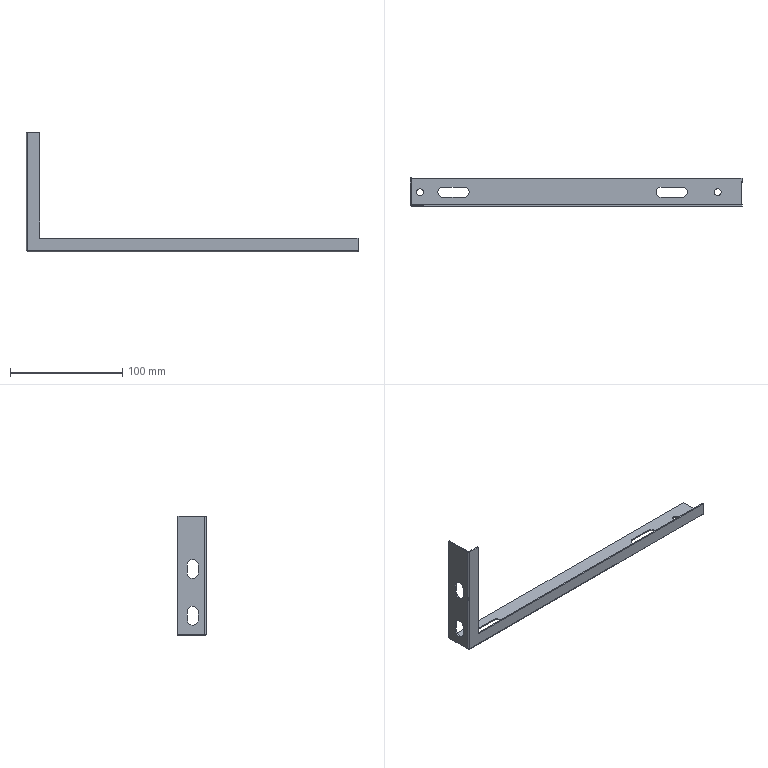Part | 1 solid | 44 faces | box 296 x 25 x 106.7 mm | volume 13427 mm3 | plane 28 | cylinder 16 | commonest cylinder face diameters 6 x4 9 x4 10 x4 0.4 x2 2.4 x2
STEP:
#1=CARTESIAN_POINT('',(125.7,14.5,-0.2));
#2=VERTEX_POINT('',#1);
#3=CARTESIAN_POINT('',(125.7,8.5,-0.2));
#4=VERTEX_POINT('',#3);
#5=CARTESIAN_POINT('',(125.7,11.5,-0.2));
#6=DIRECTION('',(0.,0.,1.));
#7=DIRECTION('',(0.,-1.,0.));
#8=AXIS2_PLACEMENT_3D('',#5,#6,#7);
#9=CIRCLE('',#8,3.);
#10=EDGE_CURVE('',#2,#4,#9,.T.);
#11=ORIENTED_EDGE('',*,*,#10,.T.);
#12=CARTESIAN_POINT('',(125.7,8.5,-1.2));
#13=VERTEX_POINT('',#12);
#14=CARTESIAN_POINT('',(125.7,8.5,8.8));
#15=DIRECTION('',(0.,0.,-1.));
#16=VECTOR('',#15,1000.);
#17=LINE('',#14,#16);
#18=EDGE_CURVE('',#4,#13,#17,.T.);
#19=ORIENTED_EDGE('',*,*,#18,.T.);
#20=CARTESIAN_POINT('',(125.7,14.5,-1.2));
#21=VERTEX_POINT('',#20);
#22=CARTESIAN_POINT('',(125.7,11.5,-1.2));
#23=DIRECTION('',(0.,0.,-1.));
#24=DIRECTION('',(0.,1.,0.));
#25=AXIS2_PLACEMENT_3D('',#22,#23,#24);
#26=CIRCLE('',#25,3.);
#27=EDGE_CURVE('',#13,#21,#26,.T.);
#28=ORIENTED_EDGE('',*,*,#27,.T.);
#29=CARTESIAN_POINT('',(125.7,14.5,8.8));
#30=DIRECTION('',(0.,0.,-1.));
#31=VECTOR('',#30,1000.);
#32=LINE('',#29,#31);
#33=EDGE_CURVE('',#2,#21,#32,.T.);
#34=ORIENTED_EDGE('',*,*,#33,.F.);
#35=EDGE_LOOP('',(#11,#19,#28,#34));
#36=FACE_OUTER_BOUND('',#35,.T.);
#37=CARTESIAN_POINT('',(125.7,11.5,8.8));
#38=DIRECTION('',(0.,0.,-1.));
#39=DIRECTION('',(0.,1.,0.));
#40=AXIS2_PLACEMENT_3D('',#37,#38,#39);
#41=CYLINDRICAL_SURFACE('',#40,3.);
#42=ADVANCED_FACE('',(#36),#41,.F.);
#43=CARTESIAN_POINT('',(-139.8,14.5,-0.2));
#44=VERTEX_POINT('',#43);
#45=CARTESIAN_POINT('',(-139.8,8.5,-0.2));
#46=VERTEX_POINT('',#45);
#47=CARTESIAN_POINT('',(-139.8,11.5,-0.2));
#48=DIRECTION('',(0.,0.,1.));
#49=DIRECTION('',(0.,-1.,0.));
#50=AXIS2_PLACEMENT_3D('',#47,#48,#49);
#51=CIRCLE('',#50,3.);
#52=EDGE_CURVE('',#44,#46,#51,.T.);
#53=ORIENTED_EDGE('',*,*,#52,.T.);
#54=CARTESIAN_POINT('',(-139.8,8.5,-1.2));
#55=VERTEX_POINT('',#54);
#56=CARTESIAN_POINT('',(-139.8,8.5,8.8));
#57=DIRECTION('',(0.,0.,-1.));
#58=VECTOR('',#57,1000.);
#59=LINE('',#56,#58);
#60=EDGE_CURVE('',#46,#55,#59,.T.);
#61=ORIENTED_EDGE('',*,*,#60,.T.);
#62=CARTESIAN_POINT('',(-139.8,14.5,-1.2));
#63=VERTEX_POINT('',#62);
#64=CARTESIAN_POINT('',(-139.8,11.5,-1.2));
#65=DIRECTION('',(0.,0.,-1.));
#66=DIRECTION('',(0.,1.,0.));
#67=AXIS2_PLACEMENT_3D('',#64,#65,#66);
#68=CIRCLE('',#67,3.);
#69=EDGE_CURVE('',#55,#63,#68,.T.);
#70=ORIENTED_EDGE('',*,*,#69,.T.);
#71=CARTESIAN_POINT('',(-139.8,14.5,8.8));
#72=DIRECTION('',(0.,0.,-1.));
#73=VECTOR('',#72,1000.);
#74=LINE('',#71,#73);
#75=EDGE_CURVE('',#44,#63,#74,.T.);
#76=ORIENTED_EDGE('',*,*,#75,.F.);
#77=EDGE_LOOP('',(#53,#61,#70,#76));
#78=FACE_OUTER_BOUND('',#77,.T.);
#79=CARTESIAN_POINT('',(-139.8,11.5,8.8));
#80=DIRECTION('',(0.,0.,-1.));
#81=DIRECTION('',(0.,1.,0.));
#82=AXIS2_PLACEMENT_3D('',#79,#80,#81);
#83=CYLINDRICAL_SURFACE('',#82,3.);
#84=ADVANCED_FACE('',(#78),#83,.F.);
#85=CARTESIAN_POINT('',(147.4,-1.,11.));
#86=VERTEX_POINT('',#85);
#87=CARTESIAN_POINT('',(-136.4,-1.,11.));
#88=VERTEX_POINT('',#87);
#89=CARTESIAN_POINT('',(-147.4,-1.,11.));
#90=DIRECTION('',(-1.,0.,0.));
#91=VECTOR('',#90,1000.);
#92=LINE('',#89,#91);
#93=EDGE_CURVE('',#86,#88,#92,.T.);
#94=ORIENTED_EDGE('',*,*,#93,.T.);
#95=CARTESIAN_POINT('',(-136.4,-1.,105.5));
#96=VERTEX_POINT('',#95);
#97=CARTESIAN_POINT('',(-136.4,-1.,105.5));
#98=DIRECTION('',(0.,0.,1.));
#99=VECTOR('',#98,1000.);
#100=LINE('',#97,#99);
#101=EDGE_CURVE('',#88,#96,#100,.T.);
#102=ORIENTED_EDGE('',*,*,#101,.T.);
#103=CARTESIAN_POINT('',(-147.4,-1.,105.5));
#104=VERTEX_POINT('',#103);
#105=CARTESIAN_POINT('',(-147.4,-1.,105.5));
#106=DIRECTION('',(1.,0.,0.));
#107=VECTOR('',#106,1000.);
#108=LINE('',#105,#107);
#109=EDGE_CURVE('',#104,#96,#108,.T.);
#110=ORIENTED_EDGE('',*,*,#109,.F.);
#111=CARTESIAN_POINT('',(-147.4,-1.,0.));
#112=VERTEX_POINT('',#111);
#113=CARTESIAN_POINT('',(-147.4,-1.,105.5));
#114=DIRECTION('',(0.,0.,-1.));
#115=VECTOR('',#114,1000.);
#116=LINE('',#113,#115);
#117=EDGE_CURVE('',#104,#112,#116,.T.);
#118=ORIENTED_EDGE('',*,*,#117,.T.);
#119=CARTESIAN_POINT('',(147.4,-1.,0.));
#120=VERTEX_POINT('',#119);
#121=CARTESIAN_POINT('',(-147.4,-1.,0.));
#122=DIRECTION('',(1.,0.,0.));
#123=VECTOR('',#122,1000.);
#124=LINE('',#121,#123);
#125=EDGE_CURVE('',#112,#120,#124,.T.);
#126=ORIENTED_EDGE('',*,*,#125,.T.);
#127=CARTESIAN_POINT('',(147.4,-1.,105.5));
#128=DIRECTION('',(0.,0.,-1.));
#129=VECTOR('',#128,1000.);
#130=LINE('',#127,#129);
#131=EDGE_CURVE('',#86,#120,#130,.T.);
#132=ORIENTED_EDGE('',*,*,#131,.F.);
#133=EDGE_LOOP('',(#94,#102,#110,#118,#126,#132));
#134=FACE_OUTER_BOUND('',#133,.T.);
#135=CARTESIAN_POINT('',(-147.4,-1.,105.5));
#136=DIRECTION('',(0.,1.,0.));
#137=DIRECTION('',(-1.,0.,0.));
#138=AXIS2_PLACEMENT_3D('',#135,#136,#137);
#139=PLANE('',#138);
#140=ADVANCED_FACE('',(#134),#139,.F.);
#141=CARTESIAN_POINT('',(147.4,0.,11.));
#142=VERTEX_POINT('',#141);
#143=CARTESIAN_POINT('',(147.4,-10.,11.));
#144=DIRECTION('',(0.,1.,0.));
#145=VECTOR('',#144,1000.);
#146=LINE('',#143,#145);
#147=EDGE_CURVE('',#86,#142,#146,.T.);
#148=ORIENTED_EDGE('',*,*,#147,.F.);
#149=ORIENTED_EDGE('',*,*,#131,.T.);
#150=CARTESIAN_POINT('',(147.4,0.,0.));
#151=VERTEX_POINT('',#150);
#152=CARTESIAN_POINT('',(147.4,0.,0.));
#153=DIRECTION('',(0.,-1.,0.));
#154=VECTOR('',#153,1000.);
#155=LINE('',#152,#154);
#156=EDGE_CURVE('',#151,#120,#155,.T.);
#157=ORIENTED_EDGE('',*,*,#156,.F.);
#158=CARTESIAN_POINT('',(147.4,0.,105.5));
#159=DIRECTION('',(0.,0.,-1.));
#160=VECTOR('',#159,1000.);
#161=LINE('',#158,#160);
#162=EDGE_CURVE('',#142,#151,#161,.T.);
#163=ORIENTED_EDGE('',*,*,#162,.F.);
#164=EDGE_LOOP('',(#148,#149,#157,#163));
#165=FACE_OUTER_BOUND('',#164,.T.);
#166=CARTESIAN_POINT('',(147.4,0.,105.5));
#167=DIRECTION('',(1.,0.,0.));
#168=DIRECTION('',(0.,0.,-1.));
#169=AXIS2_PLACEMENT_3D('',#166,#167,#168);
#170=PLANE('',#169);
#171=ADVANCED_FACE('',(#165),#170,.T.);
#172=CARTESIAN_POINT('',(-136.4,0.,11.));
#173=VERTEX_POINT('',#172);
#174=CARTESIAN_POINT('',(-136.4,0.,105.5));
#175=VERTEX_POINT('',#174);
#176=CARTESIAN_POINT('',(-136.4,0.,105.5));
#177=DIRECTION('',(0.,0.,1.));
#178=VECTOR('',#177,1000.);
#179=LINE('',#176,#178);
#180=EDGE_CURVE('',#173,#175,#179,.T.);
#181=ORIENTED_EDGE('',*,*,#180,.F.);
#182=CARTESIAN_POINT('',(147.4,0.,11.));
#183=DIRECTION('',(-1.,0.,0.));
#184=VECTOR('',#183,1000.);
#185=LINE('',#182,#184);
#186=EDGE_CURVE('',#142,#173,#185,.T.);
#187=ORIENTED_EDGE('',*,*,#186,.F.);
#188=ORIENTED_EDGE('',*,*,#162,.T.);
#189=CARTESIAN_POINT('',(-147.4,0.,0.));
#190=VERTEX_POINT('',#189);
#191=CARTESIAN_POINT('',(-147.4,0.,0.));
#192=DIRECTION('',(1.,0.,0.));
#193=VECTOR('',#192,1000.);
#194=LINE('',#191,#193);
#195=EDGE_CURVE('',#190,#151,#194,.T.);
#196=ORIENTED_EDGE('',*,*,#195,.F.);
#197=CARTESIAN_POINT('',(-147.4,0.,105.5));
#198=VERTEX_POINT('',#197);
#199=CARTESIAN_POINT('',(-147.4,0.,105.5));
#200=DIRECTION('',(0.,0.,-1.));
#201=VECTOR('',#200,1000.);
#202=LINE('',#199,#201);
#203=EDGE_CURVE('',#198,#190,#202,.T.);
#204=ORIENTED_EDGE('',*,*,#203,.F.);
#205=CARTESIAN_POINT('',(-147.4,0.,105.5));
#206=DIRECTION('',(1.,0.,0.));
#207=VECTOR('',#206,1000.);
#208=LINE('',#205,#207);
#209=EDGE_CURVE('',#198,#175,#208,.T.);
#210=ORIENTED_EDGE('',*,*,#209,.T.);
#211=EDGE_LOOP('',(#181,#187,#188,#196,#204,#210));
#212=FACE_OUTER_BOUND('',#211,.T.);
#213=CARTESIAN_POINT('',(-147.4,0.,105.5));
#214=DIRECTION('',(0.,1.,0.));
#215=DIRECTION('',(-1.,0.,0.));
#216=AXIS2_PLACEMENT_3D('',#213,#214,#215);
#217=PLANE('',#216);
#218=ADVANCED_FACE('',(#212),#217,.T.);
#219=ORIENTED_EDGE('',*,*,#109,.T.);
#220=CARTESIAN_POINT('',(-136.4,0.,105.5));
#221=DIRECTION('',(0.,1.,0.));
#222=VECTOR('',#221,1000.);
#223=LINE('',#220,#222);
#224=EDGE_CURVE('',#96,#175,#223,.T.);
#225=ORIENTED_EDGE('',*,*,#224,.T.);
#226=ORIENTED_EDGE('',*,*,#209,.F.);
#227=CARTESIAN_POINT('',(-147.4,-1.,105.5));
#228=DIRECTION('',(0.,1.,0.));
#229=VECTOR('',#228,1000.);
#230=LINE('',#227,#229);
#231=EDGE_CURVE('',#104,#198,#230,.T.);
#232=ORIENTED_EDGE('',*,*,#231,.F.);
#233=EDGE_LOOP('',(#219,#225,#226,#232));
#234=FACE_OUTER_BOUND('',#233,.T.);
#235=CARTESIAN_POINT('',(0.,0.,105.5));
#236=DIRECTION('',(0.,0.,-1.));
#237=DIRECTION('',(-1.,0.,0.));
#238=AXIS2_PLACEMENT_3D('',#235,#236,#237);
#239=PLANE('',#238);
#240=ADVANCED_FACE('',(#234),#239,.F.);
#241=ORIENTED_EDGE('',*,*,#147,.T.);
#242=ORIENTED_EDGE('',*,*,#186,.T.);
#243=CARTESIAN_POINT('',(-136.4,-10.,11.));
#244=DIRECTION('',(0.,1.,0.));
#245=VECTOR('',#244,1000.);
#246=LINE('',#243,#245);
#247=EDGE_CURVE('',#88,#173,#246,.T.);
#248=ORIENTED_EDGE('',*,*,#247,.F.);
#249=ORIENTED_EDGE('',*,*,#93,.F.);
#250=EDGE_LOOP('',(#241,#242,#248,#249));
#251=FACE_OUTER_BOUND('',#250,.T.);
#252=CARTESIAN_POINT('',(147.4,-10.,11.));
#253=DIRECTION('',(0.,0.,-1.));
#254=DIRECTION('',(-1.,0.,0.));
#255=AXIS2_PLACEMENT_3D('',#252,#253,#254);
#256=PLANE('',#255);
#257=ADVANCED_FACE('',(#251),#256,.F.);
#258=ORIENTED_EDGE('',*,*,#247,.T.);
#259=ORIENTED_EDGE('',*,*,#180,.T.);
#260=ORIENTED_EDGE('',*,*,#224,.F.);
#261=ORIENTED_EDGE('',*,*,#101,.F.);
#262=EDGE_LOOP('',(#258,#259,#260,#261));
#263=FACE_OUTER_BOUND('',#262,.T.);
#264=CARTESIAN_POINT('',(-136.4,-10.,105.5));
#265=DIRECTION('',(-1.,0.,0.));
#266=DIRECTION('',(0.,0.,1.));
#267=AXIS2_PLACEMENT_3D('',#264,#265,#266);
#268=PLANE('',#267);
#269=ADVANCED_FACE('',(#263),#268,.F.);
#270=CARTESIAN_POINT('',(147.4,0.2,-0.2));
#271=VERTEX_POINT('',#270);
#272=CARTESIAN_POINT('',(147.4,0.2,-1.2));
#273=VERTEX_POINT('',#272);
#274=CARTESIAN_POINT('',(147.4,0.2,-1.2));
#275=DIRECTION('',(0.,0.,-1.));
#276=VECTOR('',#275,1000.);
#277=LINE('',#274,#276);
#278=EDGE_CURVE('',#271,#273,#277,.T.);
#279=ORIENTED_EDGE('',*,*,#278,.F.);
#280=CARTESIAN_POINT('',(147.4,0.2,0.));
#281=DIRECTION('',(1.,0.,0.));
#282=DIRECTION('',(0.,-1.,0.));
#283=AXIS2_PLACEMENT_3D('',#280,#281,#282);
#284=CIRCLE('',#283,0.2);
#285=EDGE_CURVE('',#151,#271,#284,.T.);
#286=ORIENTED_EDGE('',*,*,#285,.F.);
#287=ORIENTED_EDGE('',*,*,#156,.T.);
#288=CARTESIAN_POINT('',(147.4,0.2,0.));
#289=DIRECTION('',(1.,0.,0.));
#290=DIRECTION('',(0.,-1.,0.));
#291=AXIS2_PLACEMENT_3D('',#288,#289,#290);
#292=CIRCLE('',#291,1.2);
#293=EDGE_CURVE('',#120,#273,#292,.T.);
#294=ORIENTED_EDGE('',*,*,#293,.T.);
#295=EDGE_LOOP('',(#279,#286,#287,#294));
#296=FACE_OUTER_BOUND('',#295,.T.);
#297=CARTESIAN_POINT('',(147.4,0.2,0.));
#298=DIRECTION('',(1.,0.,0.));
#299=DIRECTION('',(0.,1.,0.));
#300=AXIS2_PLACEMENT_3D('',#297,#298,#299);
#301=PLANE('',#300);
#302=ADVANCED_FACE('',(#296),#301,.T.);
#303=CARTESIAN_POINT('',(-147.4,0.2,-0.2));
#304=VERTEX_POINT('',#303);
#305=CARTESIAN_POINT('',(-147.4,0.2,0.));
#306=DIRECTION('',(-1.,0.,0.));
#307=DIRECTION('',(0.,-1.,0.));
#308=AXIS2_PLACEMENT_3D('',#305,#306,#307);
#309=CIRCLE('',#308,0.2);
#310=EDGE_CURVE('',#304,#190,#309,.T.);
#311=ORIENTED_EDGE('',*,*,#310,.F.);
#312=CARTESIAN_POINT('',(-147.4,0.2,-1.2));
#313=VERTEX_POINT('',#312);
#314=CARTESIAN_POINT('',(-147.4,0.2,-0.2));
#315=DIRECTION('',(0.,0.,-1.));
#316=VECTOR('',#315,1000.);
#317=LINE('',#314,#316);
#318=EDGE_CURVE('',#304,#313,#317,.T.);
#319=ORIENTED_EDGE('',*,*,#318,.T.);
#320=CARTESIAN_POINT('',(-147.4,0.2,0.));
#321=DIRECTION('',(-1.,0.,0.));
#322=DIRECTION('',(0.,-1.,0.));
#323=AXIS2_PLACEMENT_3D('',#320,#321,#322);
#324=CIRCLE('',#323,1.2);
#325=EDGE_CURVE('',#313,#112,#324,.T.);
#326=ORIENTED_EDGE('',*,*,#325,.T.);
#327=CARTESIAN_POINT('',(-147.4,-1.,0.));
#328=DIRECTION('',(0.,1.,0.));
#329=VECTOR('',#328,1000.);
#330=LINE('',#327,#329);
#331=EDGE_CURVE('',#112,#190,#330,.T.);
#332=ORIENTED_EDGE('',*,*,#331,.T.);
#333=EDGE_LOOP('',(#311,#319,#326,#332));
#334=FACE_OUTER_BOUND('',#333,.T.);
#335=CARTESIAN_POINT('',(-147.4,0.2,0.));
#336=DIRECTION('',(1.,0.,0.));
#337=DIRECTION('',(0.,1.,0.));
#338=AXIS2_PLACEMENT_3D('',#335,#336,#337);
#339=PLANE('',#338);
#340=ADVANCED_FACE('',(#334),#339,.F.);
#341=ORIENTED_EDGE('',*,*,#125,.F.);
#342=ORIENTED_EDGE('',*,*,#325,.F.);
#343=CARTESIAN_POINT('',(147.4,0.2,-1.2));
#344=DIRECTION('',(1.,0.,0.));
#345=VECTOR('',#344,1000.);
#346=LINE('',#343,#345);
#347=EDGE_CURVE('',#313,#273,#346,.T.);
#348=ORIENTED_EDGE('',*,*,#347,.T.);
#349=ORIENTED_EDGE('',*,*,#293,.F.);
#350=EDGE_LOOP('',(#341,#342,#348,#349));
#351=FACE_OUTER_BOUND('',#350,.T.);
#352=CARTESIAN_POINT('',(-147.4,0.2,0.));
#353=DIRECTION('',(-1.,0.,0.));
#354=DIRECTION('',(0.,0.,-1.));
#355=AXIS2_PLACEMENT_3D('',#352,#353,#354);
#356=CYLINDRICAL_SURFACE('',#355,1.2);
#357=ADVANCED_FACE('',(#351),#356,.T.);
#358=ORIENTED_EDGE('',*,*,#195,.T.);
#359=ORIENTED_EDGE('',*,*,#285,.T.);
#360=CARTESIAN_POINT('',(147.4,0.2,-0.2));
#361=DIRECTION('',(-1.,0.,0.));
#362=VECTOR('',#361,1000.);
#363=LINE('',#360,#362);
#364=EDGE_CURVE('',#271,#304,#363,.T.);
#365=ORIENTED_EDGE('',*,*,#364,.T.);
#366=ORIENTED_EDGE('',*,*,#310,.T.);
#367=EDGE_LOOP('',(#358,#359,#365,#366));
#368=FACE_OUTER_BOUND('',#367,.T.);
#369=CARTESIAN_POINT('',(-147.4,0.2,0.));
#370=DIRECTION('',(-1.,0.,0.));
#371=DIRECTION('',(0.,0.,-1.));
#372=AXIS2_PLACEMENT_3D('',#369,#370,#371);
#373=CYLINDRICAL_SURFACE('',#372,0.2);
#374=ADVANCED_FACE('',(#368),#373,.F.);
#375=ORIENTED_EDGE('',*,*,#318,.F.);
#376=CARTESIAN_POINT('',(-147.4,24.,-0.2));
#377=VERTEX_POINT('',#376);
#378=CARTESIAN_POINT('',(-147.4,24.,-0.2));
#379=DIRECTION('',(0.,1.,0.));
#380=VECTOR('',#379,1000.);
#381=LINE('',#378,#380);
#382=EDGE_CURVE('',#304,#377,#381,.T.);
#383=ORIENTED_EDGE('',*,*,#382,.T.);
#384=CARTESIAN_POINT('',(-147.4,24.,-1.2));
#385=VERTEX_POINT('',#384);
#386=CARTESIAN_POINT('',(-147.4,24.,-1.2));
#387=DIRECTION('',(0.,0.,1.));
#388=VECTOR('',#387,1000.);
#389=LINE('',#386,#388);
#390=EDGE_CURVE('',#385,#377,#389,.T.);
#391=ORIENTED_EDGE('',*,*,#390,.F.);
#392=CARTESIAN_POINT('',(-147.4,0.,-1.2));
#393=DIRECTION('',(0.,1.,0.));
#394=VECTOR('',#393,1000.);
#395=LINE('',#392,#394);
#396=EDGE_CURVE('',#313,#385,#395,.T.);
#397=ORIENTED_EDGE('',*,*,#396,.F.);
#398=EDGE_LOOP('',(#375,#383,#391,#397));
#399=FACE_OUTER_BOUND('',#398,.T.);
#400=CARTESIAN_POINT('',(-147.4,24.,-1.2));
#401=DIRECTION('',(1.,0.,0.));
#402=DIRECTION('',(0.,0.,-1.));
#403=AXIS2_PLACEMENT_3D('',#400,#401,#402);
#404=PLANE('',#403);
#405=ADVANCED_FACE('',(#399),#404,.F.);
#406=ORIENTED_EDGE('',*,*,#278,.T.);
#407=CARTESIAN_POINT('',(147.4,24.,-1.2));
#408=VERTEX_POINT('',#407);
#409=CARTESIAN_POINT('',(147.4,0.,-1.2));
#410=DIRECTION('',(0.,-1.,0.));
#411=VECTOR('',#410,1000.);
#412=LINE('',#409,#411);
#413=EDGE_CURVE('',#408,#273,#412,.T.);
#414=ORIENTED_EDGE('',*,*,#413,.F.);
#415=CARTESIAN_POINT('',(147.4,24.,-0.2));
#416=VERTEX_POINT('',#415);
#417=CARTESIAN_POINT('',(147.4,24.,-1.2));
#418=DIRECTION('',(0.,0.,1.));
#419=VECTOR('',#418,1000.);
#420=LINE('',#417,#419);
#421=EDGE_CURVE('',#408,#416,#420,.T.);
#422=ORIENTED_EDGE('',*,*,#421,.T.);
#423=CARTESIAN_POINT('',(147.4,0.,-0.2));
#424=DIRECTION('',(0.,-1.,0.));
#425=VECTOR('',#424,1000.);
#426=LINE('',#423,#425);
#427=EDGE_CURVE('',#416,#271,#426,.T.);
#428=ORIENTED_EDGE('',*,*,#427,.T.);
#429=EDGE_LOOP('',(#406,#414,#422,#428));
#430=FACE_OUTER_BOUND('',#429,.T.);
#431=CARTESIAN_POINT('',(147.4,0.,-1.2));
#432=DIRECTION('',(-1.,0.,0.));
#433=DIRECTION('',(0.,0.,1.));
#434=AXIS2_PLACEMENT_3D('',#431,#432,#433);
#435=PLANE('',#434);
#436=ADVANCED_FACE('',(#430),#435,.F.);
#437=CARTESIAN_POINT('',(125.7,11.5,-1.2));
#438=DIRECTION('',(0.,0.,-1.));
#439=DIRECTION('',(0.,1.,0.));
#440=AXIS2_PLACEMENT_3D('',#437,#438,#439);
#441=CIRCLE('',#440,3.);
#442=EDGE_CURVE('',#21,#13,#441,.T.);
#443=ORIENTED_EDGE('',*,*,#442,.F.);
#444=ORIENTED_EDGE('',*,*,#27,.F.);
#445=EDGE_LOOP('',(#443,#444));
#446=FACE_BOUND('',#445,.T.);
#447=CARTESIAN_POINT('',(-139.8,11.5,-1.2));
#448=DIRECTION('',(0.,0.,-1.));
#449=DIRECTION('',(0.,1.,0.));
#450=AXIS2_PLACEMENT_3D('',#447,#448,#449);
#451=CIRCLE('',#450,3.);
#452=EDGE_CURVE('',#63,#55,#451,.T.);
#453=ORIENTED_EDGE('',*,*,#452,.F.);
#454=ORIENTED_EDGE('',*,*,#69,.F.);
#455=EDGE_LOOP('',(#453,#454));
#456=FACE_BOUND('',#455,.T.);
#457=CARTESIAN_POINT('',(75.2,16.,-1.2));
#458=VERTEX_POINT('',#457);
#459=CARTESIAN_POINT('',(94.2,16.,-1.2));
#460=VERTEX_POINT('',#459);
#461=CARTESIAN_POINT('',(75.2,16.,-1.2));
#462=DIRECTION('',(1.,0.,0.));
#463=VECTOR('',#462,1000.);
#464=LINE('',#461,#463);
#465=EDGE_CURVE('',#458,#460,#464,.T.);
#466=ORIENTED_EDGE('',*,*,#465,.F.);
#467=CARTESIAN_POINT('',(75.2,7.,-1.2));
#468=VERTEX_POINT('',#467);
#469=CARTESIAN_POINT('',(75.2,11.5,-1.2));
#470=DIRECTION('',(0.,0.,-1.));
#471=DIRECTION('',(0.,1.,0.));
#472=AXIS2_PLACEMENT_3D('',#469,#470,#471);
#473=CIRCLE('',#472,4.5);
#474=EDGE_CURVE('',#468,#458,#473,.T.);
#475=ORIENTED_EDGE('',*,*,#474,.F.);
#476=CARTESIAN_POINT('',(94.2,7.,-1.2));
#477=VERTEX_POINT('',#476);
#478=CARTESIAN_POINT('',(75.2,7.,-1.2));
#479=DIRECTION('',(-1.,0.,0.));
#480=VECTOR('',#479,1000.);
#481=LINE('',#478,#480);
#482=EDGE_CURVE('',#477,#468,#481,.T.);
#483=ORIENTED_EDGE('',*,*,#482,.F.);
#484=CARTESIAN_POINT('',(94.2,11.5,-1.2));
#485=DIRECTION('',(0.,0.,-1.));
#486=DIRECTION('',(0.,1.,0.));
#487=AXIS2_PLACEMENT_3D('',#484,#485,#486);
#488=CIRCLE('',#487,4.5);
#489=EDGE_CURVE('',#460,#477,#488,.T.);
#490=ORIENTED_EDGE('',*,*,#489,.F.);
#491=EDGE_LOOP('',(#466,#475,#483,#490));
#492=FACE_BOUND('',#491,.T.);
#493=CARTESIAN_POINT('',(-119.3,16.,-1.2));
#494=VERTEX_POINT('',#493);
#495=CARTESIAN_POINT('',(-100.3,16.,-1.2));
#496=VERTEX_POINT('',#495);
#497=CARTESIAN_POINT('',(-119.3,16.,-1.2));
#498=DIRECTION('',(1.,0.,0.));
#499=VECTOR('',#498,1000.);
#500=LINE('',#497,#499);
#501=EDGE_CURVE('',#494,#496,#500,.T.);
#502=ORIENTED_EDGE('',*,*,#501,.F.);
#503=CARTESIAN_POINT('',(-119.3,7.,-1.2));
#504=VERTEX_POINT('',#503);
#505=CARTESIAN_POINT('',(-119.3,11.5,-1.2));
#506=DIRECTION('',(0.,0.,-1.));
#507=DIRECTION('',(0.,1.,0.));
#508=AXIS2_PLACEMENT_3D('',#505,#506,#507);
#509=CIRCLE('',#508,4.5);
#510=EDGE_CURVE('',#504,#494,#509,.T.);
#511=ORIENTED_EDGE('',*,*,#510,.F.);
#512=CARTESIAN_POINT('',(-100.3,7.,-1.2));
#513=VERTEX_POINT('',#512);
#514=CARTESIAN_POINT('',(-119.3,7.,-1.2));
#515=DIRECTION('',(-1.,0.,0.));
#516=VECTOR('',#515,1000.);
#517=LINE('',#514,#516);
#518=EDGE_CURVE('',#513,#504,#517,.T.);
#519=ORIENTED_EDGE('',*,*,#518,.F.);
#520=CARTESIAN_POINT('',(-100.3,11.5,-1.2));
#521=DIRECTION('',(0.,0.,-1.));
#522=DIRECTION('',(0.,1.,0.));
#523=AXIS2_PLACEMENT_3D('',#520,#521,#522);
#524=CIRCLE('',#523,4.5);
#525=EDGE_CURVE('',#496,#513,#524,.T.);
#526=ORIENTED_EDGE('',*,*,#525,.F.);
#527=EDGE_LOOP('',(#502,#511,#519,#526));
#528=FACE_BOUND('',#527,.T.);
#529=ORIENTED_EDGE('',*,*,#347,.F.);
#530=ORIENTED_EDGE('',*,*,#396,.T.);
#531=CARTESIAN_POINT('',(0.,24.,-1.2));
#532=DIRECTION('',(1.,0.,0.));
#533=VECTOR('',#532,1000.);
#534=LINE('',#531,#533);
#535=EDGE_CURVE('',#385,#408,#534,.T.);
#536=ORIENTED_EDGE('',*,*,#535,.T.);
#537=ORIENTED_EDGE('',*,*,#413,.T.);
#538=EDGE_LOOP('',(#529,#530,#536,#537));
#539=FACE_OUTER_BOUND('',#538,.T.);
#540=CARTESIAN_POINT('',(0.,0.,-1.2));
#541=DIRECTION('',(0.,0.,1.));
#542=DIRECTION('',(0.,-1.,0.));
#543=AXIS2_PLACEMENT_3D('',#540,#541,#542);
#544=PLANE('',#543);
#545=ADVANCED_FACE('',(#446,#456,#492,#528,#539),#544,.F.);
#546=ORIENTED_EDGE('',*,*,#10,.F.);
#547=CARTESIAN_POINT('',(125.7,11.5,-0.2));
#548=DIRECTION('',(0.,0.,1.));
#549=DIRECTION('',(0.,-1.,0.));
#550=AXIS2_PLACEMENT_3D('',#547,#548,#549);
#551=CIRCLE('',#550,3.);
#552=EDGE_CURVE('',#4,#2,#551,.T.);
#553=ORIENTED_EDGE('',*,*,#552,.F.);
#554=EDGE_LOOP('',(#546,#553));
#555=FACE_BOUND('',#554,.T.);
#556=ORIENTED_EDGE('',*,*,#52,.F.);
#557=CARTESIAN_POINT('',(-139.8,11.5,-0.2));
#558=DIRECTION('',(0.,0.,1.));
#559=DIRECTION('',(0.,-1.,0.));
#560=AXIS2_PLACEMENT_3D('',#557,#558,#559);
#561=CIRCLE('',#560,3.);
#562=EDGE_CURVE('',#46,#44,#561,.T.);
#563=ORIENTED_EDGE('',*,*,#562,.F.);
#564=EDGE_LOOP('',(#556,#563));
#565=FACE_BOUND('',#564,.T.);
#566=CARTESIAN_POINT('',(75.2,16.,-0.2));
#567=VERTEX_POINT('',#566);
#568=CARTESIAN_POINT('',(75.2,7.,-0.2));
#569=VERTEX_POINT('',#568);
#570=CARTESIAN_POINT('',(75.2,11.5,-0.2));
#571=DIRECTION('',(0.,0.,1.));
#572=DIRECTION('',(0.,-1.,0.));
#573=AXIS2_PLACEMENT_3D('',#570,#571,#572);
#574=CIRCLE('',#573,4.5);
#575=EDGE_CURVE('',#567,#569,#574,.T.);
#576=ORIENTED_EDGE('',*,*,#575,.F.);
#577=CARTESIAN_POINT('',(94.2,16.,-0.2));
#578=VERTEX_POINT('',#577);
#579=CARTESIAN_POINT('',(0.,16.,-0.2));
#580=DIRECTION('',(-1.,0.,0.));
#581=VECTOR('',#580,1000.);
#582=LINE('',#579,#581);
#583=EDGE_CURVE('',#578,#567,#582,.T.);
#584=ORIENTED_EDGE('',*,*,#583,.F.);
#585=CARTESIAN_POINT('',(94.2,7.,-0.2));
#586=VERTEX_POINT('',#585);
#587=CARTESIAN_POINT('',(94.2,11.5,-0.2));
#588=DIRECTION('',(0.,0.,1.));
#589=DIRECTION('',(0.,-1.,0.));
#590=AXIS2_PLACEMENT_3D('',#587,#588,#589);
#591=CIRCLE('',#590,4.5);
#592=EDGE_CURVE('',#586,#578,#591,.T.);
#593=ORIENTED_EDGE('',*,*,#592,.F.);
#594=CARTESIAN_POINT('',(0.,7.,-0.2));
#595=DIRECTION('',(1.,0.,0.));
#596=VECTOR('',#595,1000.);
#597=LINE('',#594,#596);
#598=EDGE_CURVE('',#569,#586,#597,.T.);
#599=ORIENTED_EDGE('',*,*,#598,.F.);
#600=EDGE_LOOP('',(#576,#584,#593,#599));
#601=FACE_BOUND('',#600,.T.);
#602=CARTESIAN_POINT('',(-119.3,16.,-0.2));
#603=VERTEX_POINT('',#602);
#604=CARTESIAN_POINT('',(-119.3,7.,-0.2));
#605=VERTEX_POINT('',#604);
#606=CARTESIAN_POINT('',(-119.3,11.5,-0.2));
#607=DIRECTION('',(0.,0.,1.));
#608=DIRECTION('',(0.,-1.,0.));
#609=AXIS2_PLACEMENT_3D('',#606,#607,#608);
#610=CIRCLE('',#609,4.5);
#611=EDGE_CURVE('',#603,#605,#610,.T.);
#612=ORIENTED_EDGE('',*,*,#611,.F.);
#613=CARTESIAN_POINT('',(-100.3,16.,-0.2));
#614=VERTEX_POINT('',#613);
#615=CARTESIAN_POINT('',(0.,16.,-0.2));
#616=DIRECTION('',(-1.,0.,0.));
#617=VECTOR('',#616,1000.);
#618=LINE('',#615,#617);
#619=EDGE_CURVE('',#614,#603,#618,.T.);
#620=ORIENTED_EDGE('',*,*,#619,.F.);
#621=CARTESIAN_POINT('',(-100.3,7.,-0.2));
#622=VERTEX_POINT('',#621);
#623=CARTESIAN_POINT('',(-100.3,11.5,-0.2));
#624=DIRECTION('',(0.,0.,1.));
#625=DIRECTION('',(0.,-1.,0.));
#626=AXIS2_PLACEMENT_3D('',#623,#624,#625);
#627=CIRCLE('',#626,4.5);
#628=EDGE_CURVE('',#622,#614,#627,.T.);
#629=ORIENTED_EDGE('',*,*,#628,.F.);
#630=CARTESIAN_POINT('',(0.,7.,-0.2));
#631=DIRECTION('',(1.,0.,0.));
#632=VECTOR('',#631,1000.);
#633=LINE('',#630,#632);
#634=EDGE_CURVE('',#605,#622,#633,.T.);
#635=ORIENTED_EDGE('',*,*,#634,.F.);
#636=EDGE_LOOP('',(#612,#620,#629,#635));
#637=FACE_BOUND('',#636,.T.);
#638=ORIENTED_EDGE('',*,*,#382,.F.);
#639=ORIENTED_EDGE('',*,*,#364,.F.);
#640=ORIENTED_EDGE('',*,*,#427,.F.);
#641=CARTESIAN_POINT('',(147.4,24.,-0.2));
#642=DIRECTION('',(1.,0.,0.));
#643=VECTOR('',#642,1000.);
#644=LINE('',#641,#643);
#645=EDGE_CURVE('',#377,#416,#644,.T.);
#646=ORIENTED_EDGE('',*,*,#645,.F.);
#647=EDGE_LOOP('',(#638,#639,#640,#646));
#648=FACE_OUTER_BOUND('',#647,.T.);
#649=CARTESIAN_POINT('',(0.,0.,-0.2));
#650=DIRECTION('',(0.,0.,1.));
#651=DIRECTION('',(0.,-1.,0.));
#652=AXIS2_PLACEMENT_3D('',#649,#650,#651);
#653=PLANE('',#652);
#654=ADVANCED_FACE('',(#555,#565,#601,#637,#648),#653,.T.);
#655=ORIENTED_EDGE('',*,*,#645,.T.);
#656=ORIENTED_EDGE('',*,*,#421,.F.);
#657=ORIENTED_EDGE('',*,*,#535,.F.);
#658=ORIENTED_EDGE('',*,*,#390,.T.);
#659=EDGE_LOOP('',(#655,#656,#657,#658));
#660=FACE_OUTER_BOUND('',#659,.T.);
#661=CARTESIAN_POINT('',(147.4,24.,-1.2));
#662=DIRECTION('',(0.,-1.,0.));
#663=DIRECTION('',(0.,0.,-1.));
#664=AXIS2_PLACEMENT_3D('',#661,#662,#663);
#665=PLANE('',#664);
#666=ADVANCED_FACE('',(#660),#665,.F.);
#667=CARTESIAN_POINT('',(-147.6,0.2,0.));
#668=VERTEX_POINT('',#667);
#669=CARTESIAN_POINT('',(-148.6,0.2,0.));
#670=VERTEX_POINT('',#669);
#671=CARTESIAN_POINT('',(-148.6,0.2,0.));
#672=DIRECTION('',(-1.,0.,0.));
#673=VECTOR('',#672,1000.);
#674=LINE('',#671,#673);
#675=EDGE_CURVE('',#668,#670,#674,.T.);
#676=ORIENTED_EDGE('',*,*,#675,.F.);
#677=CARTESIAN_POINT('',(-147.4,0.2,0.));
#678=DIRECTION('',(0.,0.,-1.));
#679=DIRECTION('',(0.,-1.,0.));
#680=AXIS2_PLACEMENT_3D('',#677,#678,#679);
#681=CIRCLE('',#680,0.2);
#682=EDGE_CURVE('',#190,#668,#681,.T.);
#683=ORIENTED_EDGE('',*,*,#682,.F.);
#684=ORIENTED_EDGE('',*,*,#331,.F.);
#685=CARTESIAN_POINT('',(-147.4,0.2,0.));
#686=DIRECTION('',(0.,0.,-1.));
#687=DIRECTION('',(0.,-1.,0.));
#688=AXIS2_PLACEMENT_3D('',#685,#686,#687);
#689=CIRCLE('',#688,1.2);
#690=EDGE_CURVE('',#112,#670,#689,.T.);
#691=ORIENTED_EDGE('',*,*,#690,.T.);
#692=EDGE_LOOP('',(#676,#683,#684,#691));
#693=FACE_OUTER_BOUND('',#692,.T.);
#694=CARTESIAN_POINT('',(-147.4,0.2,0.));
#695=DIRECTION('',(0.,0.,-1.));
#696=DIRECTION('',(0.,1.,0.));
#697=AXIS2_PLACEMENT_3D('',#694,#695,#696);
#698=PLANE('',#697);
#699=ADVANCED_FACE('',(#693),#698,.T.);
#700=CARTESIAN_POINT('',(-147.6,0.2,105.5));
#701=VERTEX_POINT('',#700);
#702=CARTESIAN_POINT('',(-147.4,0.2,105.5));
#703=DIRECTION('',(0.,0.,1.));
#704=DIRECTION('',(0.,-1.,0.));
#705=AXIS2_PLACEMENT_3D('',#702,#703,#704);
#706=CIRCLE('',#705,0.2);
#707=EDGE_CURVE('',#701,#198,#706,.T.);
#708=ORIENTED_EDGE('',*,*,#707,.F.);
#709=CARTESIAN_POINT('',(-148.6,0.2,105.5));
#710=VERTEX_POINT('',#709);
#711=CARTESIAN_POINT('',(-147.6,0.2,105.5));
#712=DIRECTION('',(-1.,0.,0.));
#713=VECTOR('',#712,1000.);
#714=LINE('',#711,#713);
#715=EDGE_CURVE('',#701,#710,#714,.T.);
#716=ORIENTED_EDGE('',*,*,#715,.T.);
#717=CARTESIAN_POINT('',(-147.4,0.2,105.5));
#718=DIRECTION('',(0.,0.,1.));
#719=DIRECTION('',(0.,-1.,0.));
#720=AXIS2_PLACEMENT_3D('',#717,#718,#719);
#721=CIRCLE('',#720,1.2);
#722=EDGE_CURVE('',#710,#104,#721,.T.);
#723=ORIENTED_EDGE('',*,*,#722,.T.);
#724=ORIENTED_EDGE('',*,*,#231,.T.);
#725=EDGE_LOOP('',(#708,#716,#723,#724));
#726=FACE_OUTER_BOUND('',#725,.T.);
#727=CARTESIAN_POINT('',(-147.4,0.2,105.5));
#728=DIRECTION('',(0.,0.,-1.));
#729=DIRECTION('',(0.,1.,0.));
#730=AXIS2_PLACEMENT_3D('',#727,#728,#729);
#731=PLANE('',#730);
#732=ADVANCED_FACE('',(#726),#731,.F.);
#733=ORIENTED_EDGE('',*,*,#117,.F.);
#734=ORIENTED_EDGE('',*,*,#722,.F.);
#735=CARTESIAN_POINT('',(-148.6,0.2,0.));
#736=DIRECTION('',(0.,0.,-1.));
#737=VECTOR('',#736,1000.);
#738=LINE('',#735,#737);
#739=EDGE_CURVE('',#710,#670,#738,.T.);
#740=ORIENTED_EDGE('',*,*,#739,.T.);
#741=ORIENTED_EDGE('',*,*,#690,.F.);
#742=EDGE_LOOP('',(#733,#734,#740,#741));
#743=FACE_OUTER_BOUND('',#742,.T.);
#744=CARTESIAN_POINT('',(-147.4,0.2,105.5));
#745=DIRECTION('',(0.,0.,1.));
#746=DIRECTION('',(-1.,0.,0.));
#747=AXIS2_PLACEMENT_3D('',#744,#745,#746);
#748=CYLINDRICAL_SURFACE('',#747,1.2);
#749=ADVANCED_FACE('',(#743),#748,.T.);
#750=ORIENTED_EDGE('',*,*,#203,.T.);
#751=ORIENTED_EDGE('',*,*,#682,.T.);
#752=CARTESIAN_POINT('',(-147.6,0.2,0.));
#753=DIRECTION('',(0.,0.,1.));
#754=VECTOR('',#753,1000.);
#755=LINE('',#752,#754);
#756=EDGE_CURVE('',#668,#701,#755,.T.);
#757=ORIENTED_EDGE('',*,*,#756,.T.);
#758=ORIENTED_EDGE('',*,*,#707,.T.);
#759=EDGE_LOOP('',(#750,#751,#757,#758));
#760=FACE_OUTER_BOUND('',#759,.T.);
#761=CARTESIAN_POINT('',(-147.4,0.2,105.5));
#762=DIRECTION('',(0.,0.,1.));
#763=DIRECTION('',(-1.,0.,0.));
#764=AXIS2_PLACEMENT_3D('',#761,#762,#763);
#765=CYLINDRICAL_SURFACE('',#764,0.2);
#766=ADVANCED_FACE('',(#760),#765,.F.);
#767=ORIENTED_EDGE('',*,*,#715,.F.);
#768=CARTESIAN_POINT('',(-147.6,24.,105.5));
#769=VERTEX_POINT('',#768);
#770=CARTESIAN_POINT('',(-147.6,24.,105.5));
#771=DIRECTION('',(0.,1.,0.));
#772=VECTOR('',#771,1000.);
#773=LINE('',#770,#772);
#774=EDGE_CURVE('',#701,#769,#773,.T.);
#775=ORIENTED_EDGE('',*,*,#774,.T.);
#776=CARTESIAN_POINT('',(-148.6,24.,105.5));
#777=VERTEX_POINT('',#776);
#778=CARTESIAN_POINT('',(-148.6,24.,105.5));
#779=DIRECTION('',(1.,0.,0.));
#780=VECTOR('',#779,1000.);
#781=LINE('',#778,#780);
#782=EDGE_CURVE('',#777,#769,#781,.T.);
#783=ORIENTED_EDGE('',*,*,#782,.F.);
#784=CARTESIAN_POINT('',(-148.6,0.,105.5));
#785=DIRECTION('',(0.,1.,0.));
#786=VECTOR('',#785,1000.);
#787=LINE('',#784,#786);
#788=EDGE_CURVE('',#710,#777,#787,.T.);
#789=ORIENTED_EDGE('',*,*,#788,.F.);
#790=EDGE_LOOP('',(#767,#775,#783,#789));
#791=FACE_OUTER_BOUND('',#790,.T.);
#792=CARTESIAN_POINT('',(-148.6,24.,105.5));
#793=DIRECTION('',(0.,0.,-1.));
#794=DIRECTION('',(0.,1.,0.));
#795=AXIS2_PLACEMENT_3D('',#792,#793,#794);
#796=PLANE('',#795);
#797=ADVANCED_FACE('',(#791),#796,.F.);
#798=ORIENTED_EDGE('',*,*,#675,.T.);
#799=CARTESIAN_POINT('',(-148.6,24.,0.));
#800=VERTEX_POINT('',#799);
#801=CARTESIAN_POINT('',(-148.6,0.,0.));
#802=DIRECTION('',(0.,-1.,0.));
#803=VECTOR('',#802,1000.);
#804=LINE('',#801,#803);
#805=EDGE_CURVE('',#800,#670,#804,.T.);
#806=ORIENTED_EDGE('',*,*,#805,.F.);
#807=CARTESIAN_POINT('',(-147.6,24.,0.));
#808=VERTEX_POINT('',#807);
#809=CARTESIAN_POINT('',(-148.6,24.,0.));
#810=DIRECTION('',(1.,0.,0.));
#811=VECTOR('',#810,1000.);
#812=LINE('',#809,#811);
#813=EDGE_CURVE('',#800,#808,#812,.T.);
#814=ORIENTED_EDGE('',*,*,#813,.T.);
#815=CARTESIAN_POINT('',(-147.6,0.,0.));
#816=DIRECTION('',(0.,-1.,0.));
#817=VECTOR('',#816,1000.);
#818=LINE('',#815,#817);
#819=EDGE_CURVE('',#808,#668,#818,.T.);
#820=ORIENTED_EDGE('',*,*,#819,.T.);
#821=EDGE_LOOP('',(#798,#806,#814,#820));
#822=FACE_OUTER_BOUND('',#821,.T.);
#823=CARTESIAN_POINT('',(-148.6,0.,0.));
#824=DIRECTION('',(0.,0.,1.));
#825=DIRECTION('',(0.,-1.,0.));
#826=AXIS2_PLACEMENT_3D('',#823,#824,#825);
#827=PLANE('',#826);
#828=ADVANCED_FACE('',(#822),#827,.F.);
#829=CARTESIAN_POINT('',(-148.6,5.8,54.9));
#830=VERTEX_POINT('',#829);
#831=CARTESIAN_POINT('',(-148.6,5.8,61.9));
#832=VERTEX_POINT('',#831);
#833=CARTESIAN_POINT('',(-148.6,5.8,54.9));
#834=DIRECTION('',(0.,0.,1.));
#835=VECTOR('',#834,1000.);
#836=LINE('',#833,#835);
#837=EDGE_CURVE('',#830,#832,#836,.T.);
#838=ORIENTED_EDGE('',*,*,#837,.F.);
#839=CARTESIAN_POINT('',(-148.6,15.8,54.9));
#840=VERTEX_POINT('',#839);
#841=CARTESIAN_POINT('',(-148.6,10.8,54.9));
#842=DIRECTION('',(-1.,0.,0.));
#843=DIRECTION('',(0.,-1.,0.));
#844=AXIS2_PLACEMENT_3D('',#841,#842,#843);
#845=CIRCLE('',#844,5.);
#846=EDGE_CURVE('',#840,#830,#845,.T.);
#847=ORIENTED_EDGE('',*,*,#846,.F.);
#848=CARTESIAN_POINT('',(-148.6,15.8,61.9));
#849=VERTEX_POINT('',#848);
#850=CARTESIAN_POINT('',(-148.6,15.8,54.9));
#851=DIRECTION('',(0.,0.,-1.));
#852=VECTOR('',#851,1000.);
#853=LINE('',#850,#852);
#854=EDGE_CURVE('',#849,#840,#853,.T.);
#855=ORIENTED_EDGE('',*,*,#854,.F.);
#856=CARTESIAN_POINT('',(-148.6,10.8,61.9));
#857=DIRECTION('',(-1.,0.,0.));
#858=DIRECTION('',(0.,-1.,0.));
#859=AXIS2_PLACEMENT_3D('',#856,#857,#858);
#860=CIRCLE('',#859,5.);
#861=EDGE_CURVE('',#832,#849,#860,.T.);
#862=ORIENTED_EDGE('',*,*,#861,.F.);
#863=EDGE_LOOP('',(#838,#847,#855,#862));
#864=FACE_BOUND('',#863,.T.);
#865=CARTESIAN_POINT('',(-148.6,5.8,13.3));
#866=VERTEX_POINT('',#865);
#867=CARTESIAN_POINT('',(-148.6,5.8,20.3));
#868=VERTEX_POINT('',#867);
#869=CARTESIAN_POINT('',(-148.6,5.8,13.3));
#870=DIRECTION('',(0.,0.,1.));
#871=VECTOR('',#870,1000.);
#872=LINE('',#869,#871);
#873=EDGE_CURVE('',#866,#868,#872,.T.);
#874=ORIENTED_EDGE('',*,*,#873,.F.);
#875=CARTESIAN_POINT('',(-148.6,15.8,13.3));
#876=VERTEX_POINT('',#875);
#877=CARTESIAN_POINT('',(-148.6,10.8,13.3));
#878=DIRECTION('',(-1.,0.,0.));
#879=DIRECTION('',(0.,-1.,0.));
#880=AXIS2_PLACEMENT_3D('',#877,#878,#879);
#881=CIRCLE('',#880,5.);
#882=EDGE_CURVE('',#876,#866,#881,.T.);
#883=ORIENTED_EDGE('',*,*,#882,.F.);
#884=CARTESIAN_POINT('',(-148.6,15.8,20.3));
#885=VERTEX_POINT('',#884);
#886=CARTESIAN_POINT('',(-148.6,15.8,13.3));
#887=DIRECTION('',(0.,0.,-1.));
#888=VECTOR('',#887,1000.);
#889=LINE('',#886,#888);
#890=EDGE_CURVE('',#885,#876,#889,.T.);
#891=ORIENTED_EDGE('',*,*,#890,.F.);
#892=CARTESIAN_POINT('',(-148.6,10.8,20.3));
#893=DIRECTION('',(-1.,0.,0.));
#894=DIRECTION('',(0.,-1.,0.));
#895=AXIS2_PLACEMENT_3D('',#892,#893,#894);
#896=CIRCLE('',#895,5.);
#897=EDGE_CURVE('',#868,#885,#896,.T.);
#898=ORIENTED_EDGE('',*,*,#897,.F.);
#899=EDGE_LOOP('',(#874,#883,#891,#898));
#900=FACE_BOUND('',#899,.T.);
#901=ORIENTED_EDGE('',*,*,#739,.F.);
#902=ORIENTED_EDGE('',*,*,#788,.T.);
#903=CARTESIAN_POINT('',(-148.6,24.,0.));
#904=DIRECTION('',(0.,0.,-1.));
#905=VECTOR('',#904,1000.);
#906=LINE('',#903,#905);
#907=EDGE_CURVE('',#777,#800,#906,.T.);
#908=ORIENTED_EDGE('',*,*,#907,.T.);
#909=ORIENTED_EDGE('',*,*,#805,.T.);
#910=EDGE_LOOP('',(#901,#902,#908,#909));
#911=FACE_OUTER_BOUND('',#910,.T.);
#912=CARTESIAN_POINT('',(-148.6,0.,0.));
#913=DIRECTION('',(1.,0.,0.));
#914=DIRECTION('',(0.,1.,0.));
#915=AXIS2_PLACEMENT_3D('',#912,#913,#914);
#916=PLANE('',#915);
#917=ADVANCED_FACE('',(#864,#900,#911),#916,.F.);
#918=CARTESIAN_POINT('',(-147.6,5.8,54.9));
#919=VERTEX_POINT('',#918);
#920=CARTESIAN_POINT('',(-147.6,15.8,54.9));
#921=VERTEX_POINT('',#920);
#922=CARTESIAN_POINT('',(-147.6,10.8,54.9));
#923=DIRECTION('',(1.,0.,0.));
#924=DIRECTION('',(0.,1.,0.));
#925=AXIS2_PLACEMENT_3D('',#922,#923,#924);
#926=CIRCLE('',#925,5.);
#927=EDGE_CURVE('',#919,#921,#926,.T.);
#928=ORIENTED_EDGE('',*,*,#927,.F.);
#929=CARTESIAN_POINT('',(-147.6,5.8,61.9));
#930=VERTEX_POINT('',#929);
#931=CARTESIAN_POINT('',(-147.6,5.8,0.));
#932=DIRECTION('',(0.,0.,-1.));
#933=VECTOR('',#932,1000.);
#934=LINE('',#931,#933);
#935=EDGE_CURVE('',#930,#919,#934,.T.);
#936=ORIENTED_EDGE('',*,*,#935,.F.);
#937=CARTESIAN_POINT('',(-147.6,15.8,61.9));
#938=VERTEX_POINT('',#937);
#939=CARTESIAN_POINT('',(-147.6,10.8,61.9));
#940=DIRECTION('',(1.,0.,0.));
#941=DIRECTION('',(0.,1.,0.));
#942=AXIS2_PLACEMENT_3D('',#939,#940,#941);
#943=CIRCLE('',#942,5.);
#944=EDGE_CURVE('',#938,#930,#943,.T.);
#945=ORIENTED_EDGE('',*,*,#944,.F.);
#946=CARTESIAN_POINT('',(-147.6,15.8,0.));
#947=DIRECTION('',(0.,0.,1.));
#948=VECTOR('',#947,1000.);
#949=LINE('',#946,#948);
#950=EDGE_CURVE('',#921,#938,#949,.T.);
#951=ORIENTED_EDGE('',*,*,#950,.F.);
#952=EDGE_LOOP('',(#928,#936,#945,#951));
#953=FACE_BOUND('',#952,.T.);
#954=CARTESIAN_POINT('',(-147.6,5.8,13.3));
#955=VERTEX_POINT('',#954);
#956=CARTESIAN_POINT('',(-147.6,15.8,13.3));
#957=VERTEX_POINT('',#956);
#958=CARTESIAN_POINT('',(-147.6,10.8,13.3));
#959=DIRECTION('',(1.,0.,0.));
#960=DIRECTION('',(0.,1.,0.));
#961=AXIS2_PLACEMENT_3D('',#958,#959,#960);
#962=CIRCLE('',#961,5.);
#963=EDGE_CURVE('',#955,#957,#962,.T.);
#964=ORIENTED_EDGE('',*,*,#963,.F.);
#965=CARTESIAN_POINT('',(-147.6,5.8,20.3));
#966=VERTEX_POINT('',#965);
#967=CARTESIAN_POINT('',(-147.6,5.8,0.));
#968=DIRECTION('',(0.,0.,-1.));
#969=VECTOR('',#968,1000.);
#970=LINE('',#967,#969);
#971=EDGE_CURVE('',#966,#955,#970,.T.);
#972=ORIENTED_EDGE('',*,*,#971,.F.);
#973=CARTESIAN_POINT('',(-147.6,15.8,20.3));
#974=VERTEX_POINT('',#973);
#975=CARTESIAN_POINT('',(-147.6,10.8,20.3));
#976=DIRECTION('',(1.,0.,0.));
#977=DIRECTION('',(0.,1.,0.));
#978=AXIS2_PLACEMENT_3D('',#975,#976,#977);
#979=CIRCLE('',#978,5.);
#980=EDGE_CURVE('',#974,#966,#979,.T.);
#981=ORIENTED_EDGE('',*,*,#980,.F.);
#982=CARTESIAN_POINT('',(-147.6,15.8,0.));
#983=DIRECTION('',(0.,0.,1.));
#984=VECTOR('',#983,1000.);
#985=LINE('',#982,#984);
#986=EDGE_CURVE('',#957,#974,#985,.T.);
#987=ORIENTED_EDGE('',*,*,#986,.F.);
#988=EDGE_LOOP('',(#964,#972,#981,#987));
#989=FACE_BOUND('',#988,.T.);
#990=ORIENTED_EDGE('',*,*,#774,.F.);
#991=ORIENTED_EDGE('',*,*,#756,.F.);
#992=ORIENTED_EDGE('',*,*,#819,.F.);
#993=CARTESIAN_POINT('',(-147.6,24.,0.));
#994=DIRECTION('',(0.,0.,-1.));
#995=VECTOR('',#994,1000.);
#996=LINE('',#993,#995);
#997=EDGE_CURVE('',#769,#808,#996,.T.);
#998=ORIENTED_EDGE('',*,*,#997,.F.);
#999=EDGE_LOOP('',(#990,#991,#992,#998));
#1000=FACE_OUTER_BOUND('',#999,.T.);
#1001=CARTESIAN_POINT('',(-147.6,0.,0.));
#1002=DIRECTION('',(1.,0.,0.));
#1003=DIRECTION('',(0.,1.,0.));
#1004=AXIS2_PLACEMENT_3D('',#1001,#1002,#1003);
#1005=PLANE('',#1004);
#1006=ADVANCED_FACE('',(#953,#989,#1000),#1005,.T.);
#1007=ORIENTED_EDGE('',*,*,#997,.T.);
#1008=ORIENTED_EDGE('',*,*,#813,.F.);
#1009=ORIENTED_EDGE('',*,*,#907,.F.);
#1010=ORIENTED_EDGE('',*,*,#782,.T.);
#1011=EDGE_LOOP('',(#1007,#1008,#1009,#1010));
#1012=FACE_OUTER_BOUND('',#1011,.T.);
#1013=CARTESIAN_POINT('',(-148.6,24.,0.));
#1014=DIRECTION('',(0.,-1.,0.));
#1015=DIRECTION('',(1.,0.,0.));
#1016=AXIS2_PLACEMENT_3D('',#1013,#1014,#1015);
#1017=PLANE('',#1016);
#1018=ADVANCED_FACE('',(#1012),#1017,.F.);
#1019=ORIENTED_EDGE('',*,*,#611,.T.);
#1020=CARTESIAN_POINT('',(-119.3,7.,8.8));
#1021=DIRECTION('',(0.,0.,-1.));
#1022=VECTOR('',#1021,1000.);
#1023=LINE('',#1020,#1022);
#1024=EDGE_CURVE('',#605,#504,#1023,.T.);
#1025=ORIENTED_EDGE('',*,*,#1024,.T.);
#1026=ORIENTED_EDGE('',*,*,#510,.T.);
#1027=CARTESIAN_POINT('',(-119.3,16.,8.8));
#1028=DIRECTION('',(0.,0.,-1.));
#1029=VECTOR('',#1028,1000.);
#1030=LINE('',#1027,#1029);
#1031=EDGE_CURVE('',#603,#494,#1030,.T.);
#1032=ORIENTED_EDGE('',*,*,#1031,.F.);
#1033=EDGE_LOOP('',(#1019,#1025,#1026,#1032));
#1034=FACE_OUTER_BOUND('',#1033,.T.);
#1035=CARTESIAN_POINT('',(-119.3,11.5,8.8));
#1036=DIRECTION('',(0.,0.,-1.));
#1037=DIRECTION('',(0.,1.,0.));
#1038=AXIS2_PLACEMENT_3D('',#1035,#1036,#1037);
#1039=CYLINDRICAL_SURFACE('',#1038,4.5);
#1040=ADVANCED_FACE('',(#1034),#1039,.F.);
#1041=ORIENTED_EDGE('',*,*,#634,.T.);
#1042=CARTESIAN_POINT('',(-100.3,7.,8.8));
#1043=DIRECTION('',(0.,0.,-1.));
#1044=VECTOR('',#1043,1000.);
#1045=LINE('',#1042,#1044);
#1046=EDGE_CURVE('',#622,#513,#1045,.T.);
#1047=ORIENTED_EDGE('',*,*,#1046,.T.);
#1048=ORIENTED_EDGE('',*,*,#518,.T.);
#1049=ORIENTED_EDGE('',*,*,#1024,.F.);
#1050=EDGE_LOOP('',(#1041,#1047,#1048,#1049));
#1051=FACE_OUTER_BOUND('',#1050,.T.);
#1052=CARTESIAN_POINT('',(-119.3,7.,8.8));
#1053=DIRECTION('',(0.,-1.,0.));
#1054=DIRECTION('',(0.,0.,-1.));
#1055=AXIS2_PLACEMENT_3D('',#1052,#1053,#1054);
#1056=PLANE('',#1055);
#1057=ADVANCED_FACE('',(#1051),#1056,.F.);
#1058=ORIENTED_EDGE('',*,*,#628,.T.);
#1059=CARTESIAN_POINT('',(-100.3,16.,8.8));
#1060=DIRECTION('',(0.,0.,-1.));
#1061=VECTOR('',#1060,1000.);
#1062=LINE('',#1059,#1061);
#1063=EDGE_CURVE('',#614,#496,#1062,.T.);
#1064=ORIENTED_EDGE('',*,*,#1063,.T.);
#1065=ORIENTED_EDGE('',*,*,#525,.T.);
#1066=ORIENTED_EDGE('',*,*,#1046,.F.);
#1067=EDGE_LOOP('',(#1058,#1064,#1065,#1066));
#1068=FACE_OUTER_BOUND('',#1067,.T.);
#1069=CARTESIAN_POINT('',(-100.3,11.5,8.8));
#1070=DIRECTION('',(0.,0.,-1.));
#1071=DIRECTION('',(0.,1.,0.));
#1072=AXIS2_PLACEMENT_3D('',#1069,#1070,#1071);
#1073=CYLINDRICAL_SURFACE('',#1072,4.5);
#1074=ADVANCED_FACE('',(#1068),#1073,.F.);
#1075=ORIENTED_EDGE('',*,*,#619,.T.);
#1076=ORIENTED_EDGE('',*,*,#1031,.T.);
#1077=ORIENTED_EDGE('',*,*,#501,.T.);
#1078=ORIENTED_EDGE('',*,*,#1063,.F.);
#1079=EDGE_LOOP('',(#1075,#1076,#1077,#1078));
#1080=FACE_OUTER_BOUND('',#1079,.T.);
#1081=CARTESIAN_POINT('',(-119.3,16.,8.8));
#1082=DIRECTION('',(0.,1.,0.));
#1083=DIRECTION('',(0.,0.,1.));
#1084=AXIS2_PLACEMENT_3D('',#1081,#1082,#1083);
#1085=PLANE('',#1084);
#1086=ADVANCED_FACE('',(#1080),#1085,.F.);
#1087=ORIENTED_EDGE('',*,*,#575,.T.);
#1088=CARTESIAN_POINT('',(75.2,7.,8.8));
#1089=DIRECTION('',(0.,0.,-1.));
#1090=VECTOR('',#1089,1000.);
#1091=LINE('',#1088,#1090);
#1092=EDGE_CURVE('',#569,#468,#1091,.T.);
#1093=ORIENTED_EDGE('',*,*,#1092,.T.);
#1094=ORIENTED_EDGE('',*,*,#474,.T.);
#1095=CARTESIAN_POINT('',(75.2,16.,8.8));
#1096=DIRECTION('',(0.,0.,-1.));
#1097=VECTOR('',#1096,1000.);
#1098=LINE('',#1095,#1097);
#1099=EDGE_CURVE('',#567,#458,#1098,.T.);
#1100=ORIENTED_EDGE('',*,*,#1099,.F.);
#1101=EDGE_LOOP('',(#1087,#1093,#1094,#1100));
#1102=FACE_OUTER_BOUND('',#1101,.T.);
#1103=CARTESIAN_POINT('',(75.2,11.5,8.8));
#1104=DIRECTION('',(0.,0.,-1.));
#1105=DIRECTION('',(0.,1.,0.));
#1106=AXIS2_PLACEMENT_3D('',#1103,#1104,#1105);
#1107=CYLINDRICAL_SURFACE('',#1106,4.5);
#1108=ADVANCED_FACE('',(#1102),#1107,.F.);
#1109=ORIENTED_EDGE('',*,*,#598,.T.);
#1110=CARTESIAN_POINT('',(94.2,7.,8.8));
#1111=DIRECTION('',(0.,0.,-1.));
#1112=VECTOR('',#1111,1000.);
#1113=LINE('',#1110,#1112);
#1114=EDGE_CURVE('',#586,#477,#1113,.T.);
#1115=ORIENTED_EDGE('',*,*,#1114,.T.);
#1116=ORIENTED_EDGE('',*,*,#482,.T.);
#1117=ORIENTED_EDGE('',*,*,#1092,.F.);
#1118=EDGE_LOOP('',(#1109,#1115,#1116,#1117));
#1119=FACE_OUTER_BOUND('',#1118,.T.);
#1120=CARTESIAN_POINT('',(75.2,7.,8.8));
#1121=DIRECTION('',(0.,-1.,0.));
#1122=DIRECTION('',(0.,0.,-1.));
#1123=AXIS2_PLACEMENT_3D('',#1120,#1121,#1122);
#1124=PLANE('',#1123);
#1125=ADVANCED_FACE('',(#1119),#1124,.F.);
#1126=ORIENTED_EDGE('',*,*,#592,.T.);
#1127=CARTESIAN_POINT('',(94.2,16.,8.8));
#1128=DIRECTION('',(0.,0.,-1.));
#1129=VECTOR('',#1128,1000.);
#1130=LINE('',#1127,#1129);
#1131=EDGE_CURVE('',#578,#460,#1130,.T.);
#1132=ORIENTED_EDGE('',*,*,#1131,.T.);
#1133=ORIENTED_EDGE('',*,*,#489,.T.);
#1134=ORIENTED_EDGE('',*,*,#1114,.F.);
#1135=EDGE_LOOP('',(#1126,#1132,#1133,#1134));
#1136=FACE_OUTER_BOUND('',#1135,.T.);
#1137=CARTESIAN_POINT('',(94.2,11.5,8.8));
#1138=DIRECTION('',(0.,0.,-1.));
#1139=DIRECTION('',(0.,1.,0.));
#1140=AXIS2_PLACEMENT_3D('',#1137,#1138,#1139);
#1141=CYLINDRICAL_SURFACE('',#1140,4.5);
#1142=ADVANCED_FACE('',(#1136),#1141,.F.);
#1143=ORIENTED_EDGE('',*,*,#583,.T.);
#1144=ORIENTED_EDGE('',*,*,#1099,.T.);
#1145=ORIENTED_EDGE('',*,*,#465,.T.);
#1146=ORIENTED_EDGE('',*,*,#1131,.F.);
#1147=EDGE_LOOP('',(#1143,#1144,#1145,#1146));
#1148=FACE_OUTER_BOUND('',#1147,.T.);
#1149=CARTESIAN_POINT('',(75.2,16.,8.8));
#1150=DIRECTION('',(0.,1.,0.));
#1151=DIRECTION('',(0.,0.,1.));
#1152=AXIS2_PLACEMENT_3D('',#1149,#1150,#1151);
#1153=PLANE('',#1152);
#1154=ADVANCED_FACE('',(#1148),#1153,.F.);
#1155=ORIENTED_EDGE('',*,*,#60,.F.);
#1156=ORIENTED_EDGE('',*,*,#562,.T.);
#1157=ORIENTED_EDGE('',*,*,#75,.T.);
#1158=ORIENTED_EDGE('',*,*,#452,.T.);
#1159=EDGE_LOOP('',(#1155,#1156,#1157,#1158));
#1160=FACE_OUTER_BOUND('',#1159,.T.);
#1161=CARTESIAN_POINT('',(-139.8,11.5,8.8));
#1162=DIRECTION('',(0.,0.,-1.));
#1163=DIRECTION('',(0.,1.,0.));
#1164=AXIS2_PLACEMENT_3D('',#1161,#1162,#1163);
#1165=CYLINDRICAL_SURFACE('',#1164,3.);
#1166=ADVANCED_FACE('',(#1160),#1165,.F.);
#1167=ORIENTED_EDGE('',*,*,#18,.F.);
#1168=ORIENTED_EDGE('',*,*,#552,.T.);
#1169=ORIENTED_EDGE('',*,*,#33,.T.);
#1170=ORIENTED_EDGE('',*,*,#442,.T.);
#1171=EDGE_LOOP('',(#1167,#1168,#1169,#1170));
#1172=FACE_OUTER_BOUND('',#1171,.T.);
#1173=CARTESIAN_POINT('',(125.7,11.5,8.8));
#1174=DIRECTION('',(0.,0.,-1.));
#1175=DIRECTION('',(0.,1.,0.));
#1176=AXIS2_PLACEMENT_3D('',#1173,#1174,#1175);
#1177=CYLINDRICAL_SURFACE('',#1176,3.);
#1178=ADVANCED_FACE('',(#1172),#1177,.F.);
#1179=ORIENTED_EDGE('',*,*,#963,.T.);
#1180=CARTESIAN_POINT('',(-138.6,15.8,13.3));
#1181=DIRECTION('',(-1.,0.,0.));
#1182=VECTOR('',#1181,1000.);
#1183=LINE('',#1180,#1182);
#1184=EDGE_CURVE('',#957,#876,#1183,.T.);
#1185=ORIENTED_EDGE('',*,*,#1184,.T.);
#1186=ORIENTED_EDGE('',*,*,#882,.T.);
#1187=CARTESIAN_POINT('',(-138.6,5.8,13.3));
#1188=DIRECTION('',(-1.,0.,0.));
#1189=VECTOR('',#1188,1000.);
#1190=LINE('',#1187,#1189);
#1191=EDGE_CURVE('',#955,#866,#1190,.T.);
#1192=ORIENTED_EDGE('',*,*,#1191,.F.);
#1193=EDGE_LOOP('',(#1179,#1185,#1186,#1192));
#1194=FACE_OUTER_BOUND('',#1193,.T.);
#1195=CARTESIAN_POINT('',(-138.6,10.8,13.3));
#1196=DIRECTION('',(-1.,0.,0.));
#1197=DIRECTION('',(0.,-1.,0.));
#1198=AXIS2_PLACEMENT_3D('',#1195,#1196,#1197);
#1199=CYLINDRICAL_SURFACE('',#1198,5.);
#1200=ADVANCED_FACE('',(#1194),#1199,.F.);
#1201=ORIENTED_EDGE('',*,*,#986,.T.);
#1202=CARTESIAN_POINT('',(-138.6,15.8,20.3));
#1203=DIRECTION('',(-1.,0.,0.));
#1204=VECTOR('',#1203,1000.);
#1205=LINE('',#1202,#1204);
#1206=EDGE_CURVE('',#974,#885,#1205,.T.);
#1207=ORIENTED_EDGE('',*,*,#1206,.T.);
#1208=ORIENTED_EDGE('',*,*,#890,.T.);
#1209=ORIENTED_EDGE('',*,*,#1184,.F.);
#1210=EDGE_LOOP('',(#1201,#1207,#1208,#1209));
#1211=FACE_OUTER_BOUND('',#1210,.T.);
#1212=CARTESIAN_POINT('',(-138.6,15.8,13.3));
#1213=DIRECTION('',(0.,1.,0.));
#1214=DIRECTION('',(-1.,0.,0.));
#1215=AXIS2_PLACEMENT_3D('',#1212,#1213,#1214);
#1216=PLANE('',#1215);
#1217=ADVANCED_FACE('',(#1211),#1216,.F.);
#1218=ORIENTED_EDGE('',*,*,#980,.T.);
#1219=CARTESIAN_POINT('',(-138.6,5.8,20.3));
#1220=DIRECTION('',(-1.,0.,0.));
#1221=VECTOR('',#1220,1000.);
#1222=LINE('',#1219,#1221);
#1223=EDGE_CURVE('',#966,#868,#1222,.T.);
#1224=ORIENTED_EDGE('',*,*,#1223,.T.);
#1225=ORIENTED_EDGE('',*,*,#897,.T.);
#1226=ORIENTED_EDGE('',*,*,#1206,.F.);
#1227=EDGE_LOOP('',(#1218,#1224,#1225,#1226));
#1228=FACE_OUTER_BOUND('',#1227,.T.);
#1229=CARTESIAN_POINT('',(-138.6,10.8,20.3));
#1230=DIRECTION('',(-1.,0.,0.));
#1231=DIRECTION('',(0.,-1.,0.));
#1232=AXIS2_PLACEMENT_3D('',#1229,#1230,#1231);
#1233=CYLINDRICAL_SURFACE('',#1232,5.);
#1234=ADVANCED_FACE('',(#1228),#1233,.F.);
#1235=ORIENTED_EDGE('',*,*,#971,.T.);
#1236=ORIENTED_EDGE('',*,*,#1191,.T.);
#1237=ORIENTED_EDGE('',*,*,#873,.T.);
#1238=ORIENTED_EDGE('',*,*,#1223,.F.);
#1239=EDGE_LOOP('',(#1235,#1236,#1237,#1238));
#1240=FACE_OUTER_BOUND('',#1239,.T.);
#1241=CARTESIAN_POINT('',(-138.6,5.8,13.3));
#1242=DIRECTION('',(0.,-1.,0.));
#1243=DIRECTION('',(1.,0.,0.));
#1244=AXIS2_PLACEMENT_3D('',#1241,#1242,#1243);
#1245=PLANE('',#1244);
#1246=ADVANCED_FACE('',(#1240),#1245,.F.);
#1247=ORIENTED_EDGE('',*,*,#927,.T.);
#1248=CARTESIAN_POINT('',(-138.6,15.8,54.9));
#1249=DIRECTION('',(-1.,0.,0.));
#1250=VECTOR('',#1249,1000.);
#1251=LINE('',#1248,#1250);
#1252=EDGE_CURVE('',#921,#840,#1251,.T.);
#1253=ORIENTED_EDGE('',*,*,#1252,.T.);
#1254=ORIENTED_EDGE('',*,*,#846,.T.);
#1255=CARTESIAN_POINT('',(-138.6,5.8,54.9));
#1256=DIRECTION('',(-1.,0.,0.));
#1257=VECTOR('',#1256,1000.);
#1258=LINE('',#1255,#1257);
#1259=EDGE_CURVE('',#919,#830,#1258,.T.);
#1260=ORIENTED_EDGE('',*,*,#1259,.F.);
#1261=EDGE_LOOP('',(#1247,#1253,#1254,#1260));
#1262=FACE_OUTER_BOUND('',#1261,.T.);
#1263=CARTESIAN_POINT('',(-138.6,10.8,54.9));
#1264=DIRECTION('',(-1.,0.,0.));
#1265=DIRECTION('',(0.,-1.,0.));
#1266=AXIS2_PLACEMENT_3D('',#1263,#1264,#1265);
#1267=CYLINDRICAL_SURFACE('',#1266,5.);
#1268=ADVANCED_FACE('',(#1262),#1267,.F.);
#1269=ORIENTED_EDGE('',*,*,#950,.T.);
#1270=CARTESIAN_POINT('',(-138.6,15.8,61.9));
#1271=DIRECTION('',(-1.,0.,0.));
#1272=VECTOR('',#1271,1000.);
#1273=LINE('',#1270,#1272);
#1274=EDGE_CURVE('',#938,#849,#1273,.T.);
#1275=ORIENTED_EDGE('',*,*,#1274,.T.);
#1276=ORIENTED_EDGE('',*,*,#854,.T.);
#1277=ORIENTED_EDGE('',*,*,#1252,.F.);
#1278=EDGE_LOOP('',(#1269,#1275,#1276,#1277));
#1279=FACE_OUTER_BOUND('',#1278,.T.);
#1280=CARTESIAN_POINT('',(-138.6,15.8,54.9));
#1281=DIRECTION('',(0.,1.,0.));
#1282=DIRECTION('',(-1.,0.,0.));
#1283=AXIS2_PLACEMENT_3D('',#1280,#1281,#1282);
#1284=PLANE('',#1283);
#1285=ADVANCED_FACE('',(#1279),#1284,.F.);
#1286=ORIENTED_EDGE('',*,*,#944,.T.);
#1287=CARTESIAN_POINT('',(-138.6,5.8,61.9));
#1288=DIRECTION('',(-1.,0.,0.));
#1289=VECTOR('',#1288,1000.);
#1290=LINE('',#1287,#1289);
#1291=EDGE_CURVE('',#930,#832,#1290,.T.);
#1292=ORIENTED_EDGE('',*,*,#1291,.T.);
#1293=ORIENTED_EDGE('',*,*,#861,.T.);
#1294=ORIENTED_EDGE('',*,*,#1274,.F.);
#1295=EDGE_LOOP('',(#1286,#1292,#1293,#1294));
#1296=FACE_OUTER_BOUND('',#1295,.T.);
#1297=CARTESIAN_POINT('',(-138.6,10.8,61.9));
#1298=DIRECTION('',(-1.,0.,0.));
#1299=DIRECTION('',(0.,-1.,0.));
#1300=AXIS2_PLACEMENT_3D('',#1297,#1298,#1299);
#1301=CYLINDRICAL_SURFACE('',#1300,5.);
#1302=ADVANCED_FACE('',(#1296),#1301,.F.);
#1303=ORIENTED_EDGE('',*,*,#935,.T.);
#1304=ORIENTED_EDGE('',*,*,#1259,.T.);
#1305=ORIENTED_EDGE('',*,*,#837,.T.);
#1306=ORIENTED_EDGE('',*,*,#1291,.F.);
#1307=EDGE_LOOP('',(#1303,#1304,#1305,#1306));
#1308=FACE_OUTER_BOUND('',#1307,.T.);
#1309=CARTESIAN_POINT('',(-138.6,5.8,54.9));
#1310=DIRECTION('',(0.,-1.,0.));
#1311=DIRECTION('',(1.,0.,0.));
#1312=AXIS2_PLACEMENT_3D('',#1309,#1310,#1311);
#1313=PLANE('',#1312);
#1314=ADVANCED_FACE('',(#1308),#1313,.F.);
#1315=CLOSED_SHELL('',(#42,#84,#140,#171,#218,#240,#257,#269,#302,#340,#357,#374,#405,#436,#545,#654,#666,#699,#732,#749,#766,#797,#828,#917,#1006,#1018,#1040,#1057,#1074,#1086,#1108,#1125,#1142,#1154,#1166,#1178,#1200,#1217,#1234,#1246,#1268,#1285,#1302,#1314));
#1316=MANIFOLD_SOLID_BREP('',#1315);
#1317=CARTESIAN_POINT('',(0.,0.,0.));
#1318=DIRECTION('',(0.,0.,1.));
#1319=DIRECTION('',(1.,0.,0.));
#1320=AXIS2_PLACEMENT_3D('',#1317,#1318,#1319);
#1321=(LENGTH_UNIT()NAMED_UNIT(*)SI_UNIT(.MILLI.,.METRE.));
#1322=UNCERTAINTY_MEASURE_WITH_UNIT(LENGTH_MEASURE(0.00001),#1321,'','');
#1323=(NAMED_UNIT(*)PLANE_ANGLE_UNIT()SI_UNIT($,.RADIAN.));
#1324=(NAMED_UNIT(*)SI_UNIT($,.STERADIAN.)SOLID_ANGLE_UNIT());
#1325=(GEOMETRIC_REPRESENTATION_CONTEXT(3)GLOBAL_UNCERTAINTY_ASSIGNED_CONTEXT((#1322))GLOBAL_UNIT_ASSIGNED_CONTEXT((#1321,#1323,#1324))REPRESENTATION_CONTEXT('',''));
#1326=ADVANCED_BREP_SHAPE_REPRESENTATION('',(#1316,#1320),#1325);